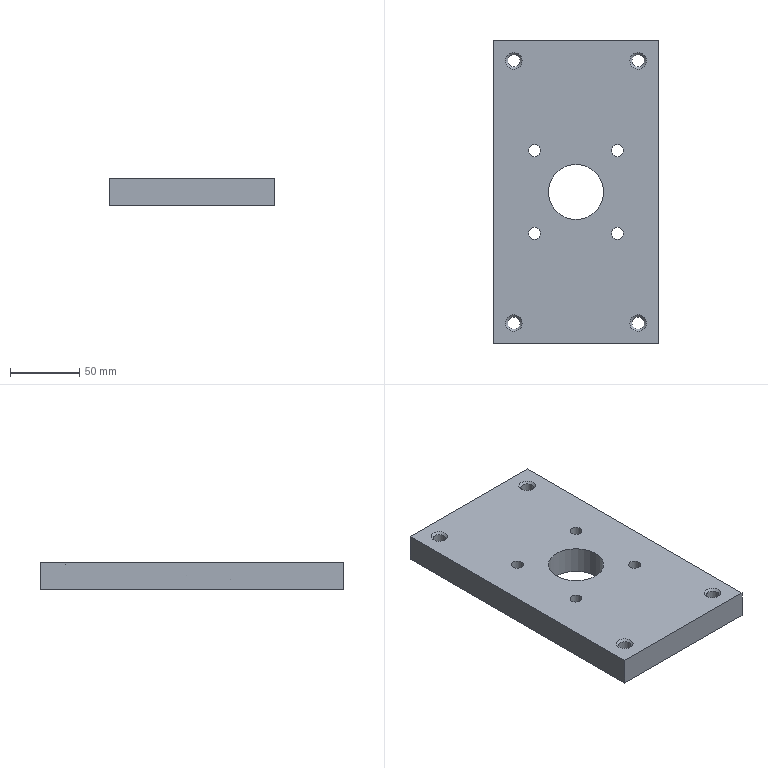Part | STEP file | YBQDJ-PD-14 | 1 solid | 27 faces | box 120 x 220 x 20 mm | volume 489101 mm3 | cylinder 13 | plane 10 | cone 4 | commonest cylinder face diameters 8.7 x4 9 x4 14 x4 40 x1